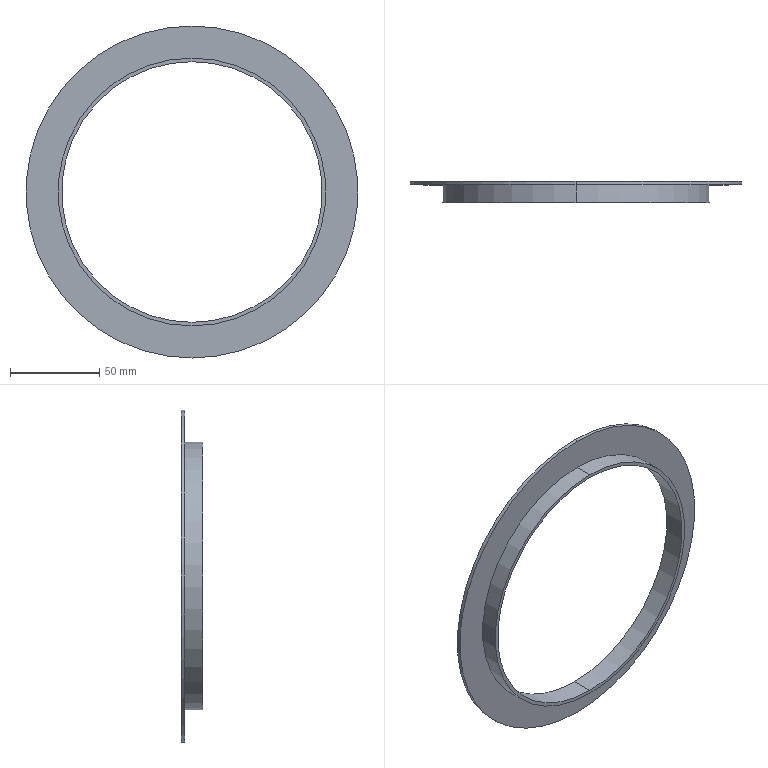Part | SolidWorks | features Extrusion 1, ICE 1 | 1 solid | 9 faces | box 186 x 12 x 186 mm | volume 30159 mm3 | cylinder 6 | plane 3 | commonest cylinder face diameters 146 x2 150 x2 186 x2
STEP:
#1=CARTESIAN_POINT('',(0.,12.,93.));
#2=VERTEX_POINT('',#1);
#3=CARTESIAN_POINT('',(0.,12.,-93.));
#4=VERTEX_POINT('',#3);
#5=CARTESIAN_POINT('',(0.,12.,0.));
#6=DIRECTION('',(0.,1.,0.));
#7=DIRECTION('',(0.,0.,1.));
#8=AXIS2_PLACEMENT_3D('',#5,#6,#7);
#9=CIRCLE('',#8,93.);
#10=EDGE_CURVE('',#2,#4,#9,.T.);
#11=ORIENTED_EDGE('',*,*,#10,.F.);
#12=CARTESIAN_POINT('',(0.,10.,93.));
#13=VERTEX_POINT('',#12);
#14=CARTESIAN_POINT('',(0.,12.,93.));
#15=DIRECTION('',(0.,-1.,0.));
#16=VECTOR('',#15,1000.);
#17=LINE('',#14,#16);
#18=EDGE_CURVE('',#2,#13,#17,.T.);
#19=ORIENTED_EDGE('',*,*,#18,.T.);
#20=CARTESIAN_POINT('',(0.,10.,-93.));
#21=VERTEX_POINT('',#20);
#22=CARTESIAN_POINT('',(0.,10.,0.));
#23=DIRECTION('',(0.,1.,0.));
#24=DIRECTION('',(0.,0.,1.));
#25=AXIS2_PLACEMENT_3D('',#22,#23,#24);
#26=CIRCLE('',#25,93.);
#27=EDGE_CURVE('',#13,#21,#26,.T.);
#28=ORIENTED_EDGE('',*,*,#27,.T.);
#29=CARTESIAN_POINT('',(0.,12.,-93.));
#30=DIRECTION('',(0.,-1.,0.));
#31=VECTOR('',#30,1000.);
#32=LINE('',#29,#31);
#33=EDGE_CURVE('',#4,#21,#32,.T.);
#34=ORIENTED_EDGE('',*,*,#33,.F.);
#35=EDGE_LOOP('',(#11,#19,#28,#34));
#36=FACE_OUTER_BOUND('',#35,.T.);
#37=CARTESIAN_POINT('',(0.,12.,0.));
#38=DIRECTION('',(0.,-1.,0.));
#39=DIRECTION('',(0.,0.,-1.));
#40=AXIS2_PLACEMENT_3D('',#37,#38,#39);
#41=CYLINDRICAL_SURFACE('',#40,93.);
#42=ADVANCED_FACE('',(#36),#41,.T.);
#43=CARTESIAN_POINT('',(0.,12.,-73.));
#44=VERTEX_POINT('',#43);
#45=CARTESIAN_POINT('',(0.,12.,73.));
#46=VERTEX_POINT('',#45);
#47=CARTESIAN_POINT('',(0.,12.,0.));
#48=DIRECTION('',(0.,1.,0.));
#49=DIRECTION('',(0.,0.,1.));
#50=AXIS2_PLACEMENT_3D('',#47,#48,#49);
#51=CIRCLE('',#50,73.);
#52=EDGE_CURVE('',#44,#46,#51,.T.);
#53=ORIENTED_EDGE('',*,*,#52,.T.);
#54=CARTESIAN_POINT('',(0.,0.,73.));
#55=VERTEX_POINT('',#54);
#56=CARTESIAN_POINT('',(0.,10.,73.));
#57=DIRECTION('',(0.,-1.,0.));
#58=VECTOR('',#57,1000.);
#59=LINE('',#56,#58);
#60=EDGE_CURVE('',#46,#55,#59,.T.);
#61=ORIENTED_EDGE('',*,*,#60,.T.);
#62=CARTESIAN_POINT('',(0.,0.,-73.));
#63=VERTEX_POINT('',#62);
#64=CARTESIAN_POINT('',(0.,0.,0.));
#65=DIRECTION('',(0.,1.,0.));
#66=DIRECTION('',(0.,0.,1.));
#67=AXIS2_PLACEMENT_3D('',#64,#65,#66);
#68=CIRCLE('',#67,73.);
#69=EDGE_CURVE('',#63,#55,#68,.T.);
#70=ORIENTED_EDGE('',*,*,#69,.F.);
#71=CARTESIAN_POINT('',(0.,10.,-73.));
#72=DIRECTION('',(0.,-1.,0.));
#73=VECTOR('',#72,1000.);
#74=LINE('',#71,#73);
#75=EDGE_CURVE('',#44,#63,#74,.T.);
#76=ORIENTED_EDGE('',*,*,#75,.F.);
#77=EDGE_LOOP('',(#53,#61,#70,#76));
#78=FACE_OUTER_BOUND('',#77,.T.);
#79=CARTESIAN_POINT('',(0.,10.,0.));
#80=DIRECTION('',(0.,-1.,0.));
#81=DIRECTION('',(0.,0.,-1.));
#82=AXIS2_PLACEMENT_3D('',#79,#80,#81);
#83=CYLINDRICAL_SURFACE('',#82,73.);
#84=ADVANCED_FACE('',(#78),#83,.F.);
#85=CARTESIAN_POINT('',(0.,10.,75.));
#86=VERTEX_POINT('',#85);
#87=CARTESIAN_POINT('',(0.,10.,-75.));
#88=VERTEX_POINT('',#87);
#89=CARTESIAN_POINT('',(0.,10.,0.));
#90=DIRECTION('',(0.,1.,0.));
#91=DIRECTION('',(0.,0.,1.));
#92=AXIS2_PLACEMENT_3D('',#89,#90,#91);
#93=CIRCLE('',#92,75.);
#94=EDGE_CURVE('',#86,#88,#93,.T.);
#95=ORIENTED_EDGE('',*,*,#94,.F.);
#96=CARTESIAN_POINT('',(0.,0.,75.));
#97=VERTEX_POINT('',#96);
#98=CARTESIAN_POINT('',(0.,10.,75.));
#99=DIRECTION('',(0.,-1.,0.));
#100=VECTOR('',#99,1000.);
#101=LINE('',#98,#100);
#102=EDGE_CURVE('',#86,#97,#101,.T.);
#103=ORIENTED_EDGE('',*,*,#102,.T.);
#104=CARTESIAN_POINT('',(0.,0.,-75.));
#105=VERTEX_POINT('',#104);
#106=CARTESIAN_POINT('',(0.,0.,0.));
#107=DIRECTION('',(0.,1.,0.));
#108=DIRECTION('',(0.,0.,1.));
#109=AXIS2_PLACEMENT_3D('',#106,#107,#108);
#110=CIRCLE('',#109,75.);
#111=EDGE_CURVE('',#97,#105,#110,.T.);
#112=ORIENTED_EDGE('',*,*,#111,.T.);
#113=CARTESIAN_POINT('',(0.,10.,-75.));
#114=DIRECTION('',(0.,-1.,0.));
#115=VECTOR('',#114,1000.);
#116=LINE('',#113,#115);
#117=EDGE_CURVE('',#88,#105,#116,.T.);
#118=ORIENTED_EDGE('',*,*,#117,.F.);
#119=EDGE_LOOP('',(#95,#103,#112,#118));
#120=FACE_OUTER_BOUND('',#119,.T.);
#121=CARTESIAN_POINT('',(0.,10.,0.));
#122=DIRECTION('',(0.,-1.,0.));
#123=DIRECTION('',(0.,0.,-1.));
#124=AXIS2_PLACEMENT_3D('',#121,#122,#123);
#125=CYLINDRICAL_SURFACE('',#124,75.);
#126=ADVANCED_FACE('',(#120),#125,.T.);
#127=CARTESIAN_POINT('',(0.,0.,0.));
#128=DIRECTION('',(0.,1.,0.));
#129=DIRECTION('',(0.,0.,1.));
#130=AXIS2_PLACEMENT_3D('',#127,#128,#129);
#131=CIRCLE('',#130,75.);
#132=EDGE_CURVE('',#105,#97,#131,.T.);
#133=ORIENTED_EDGE('',*,*,#132,.F.);
#134=ORIENTED_EDGE('',*,*,#111,.F.);
#135=EDGE_LOOP('',(#133,#134));
#136=FACE_OUTER_BOUND('',#135,.T.);
#137=ORIENTED_EDGE('',*,*,#69,.T.);
#138=CARTESIAN_POINT('',(0.,0.,0.));
#139=DIRECTION('',(0.,1.,0.));
#140=DIRECTION('',(0.,0.,1.));
#141=AXIS2_PLACEMENT_3D('',#138,#139,#140);
#142=CIRCLE('',#141,73.);
#143=EDGE_CURVE('',#55,#63,#142,.T.);
#144=ORIENTED_EDGE('',*,*,#143,.T.);
#145=EDGE_LOOP('',(#137,#144));
#146=FACE_BOUND('',#145,.T.);
#147=CARTESIAN_POINT('',(0.,0.,0.));
#148=DIRECTION('',(0.,1.,0.));
#149=DIRECTION('',(0.,0.,1.));
#150=AXIS2_PLACEMENT_3D('',#147,#148,#149);
#151=PLANE('',#150);
#152=ADVANCED_FACE('',(#136,#146),#151,.F.);
#153=ORIENTED_EDGE('',*,*,#102,.F.);
#154=CARTESIAN_POINT('',(0.,10.,0.));
#155=DIRECTION('',(0.,1.,0.));
#156=DIRECTION('',(0.,0.,1.));
#157=AXIS2_PLACEMENT_3D('',#154,#155,#156);
#158=CIRCLE('',#157,75.);
#159=EDGE_CURVE('',#88,#86,#158,.T.);
#160=ORIENTED_EDGE('',*,*,#159,.F.);
#161=ORIENTED_EDGE('',*,*,#117,.T.);
#162=ORIENTED_EDGE('',*,*,#132,.T.);
#163=EDGE_LOOP('',(#153,#160,#161,#162));
#164=FACE_OUTER_BOUND('',#163,.T.);
#165=CARTESIAN_POINT('',(0.,10.,0.));
#166=DIRECTION('',(0.,-1.,0.));
#167=DIRECTION('',(0.,0.,-1.));
#168=AXIS2_PLACEMENT_3D('',#165,#166,#167);
#169=CYLINDRICAL_SURFACE('',#168,75.);
#170=ADVANCED_FACE('',(#164),#169,.T.);
#171=ORIENTED_EDGE('',*,*,#60,.F.);
#172=CARTESIAN_POINT('',(0.,12.,0.));
#173=DIRECTION('',(0.,1.,0.));
#174=DIRECTION('',(0.,0.,1.));
#175=AXIS2_PLACEMENT_3D('',#172,#173,#174);
#176=CIRCLE('',#175,73.);
#177=EDGE_CURVE('',#46,#44,#176,.T.);
#178=ORIENTED_EDGE('',*,*,#177,.T.);
#179=ORIENTED_EDGE('',*,*,#75,.T.);
#180=ORIENTED_EDGE('',*,*,#143,.F.);
#181=EDGE_LOOP('',(#171,#178,#179,#180));
#182=FACE_OUTER_BOUND('',#181,.T.);
#183=CARTESIAN_POINT('',(0.,10.,0.));
#184=DIRECTION('',(0.,-1.,0.));
#185=DIRECTION('',(0.,0.,-1.));
#186=AXIS2_PLACEMENT_3D('',#183,#184,#185);
#187=CYLINDRICAL_SURFACE('',#186,73.);
#188=ADVANCED_FACE('',(#182),#187,.F.);
#189=CARTESIAN_POINT('',(0.,12.,0.));
#190=DIRECTION('',(0.,1.,0.));
#191=DIRECTION('',(0.,0.,1.));
#192=AXIS2_PLACEMENT_3D('',#189,#190,#191);
#193=CIRCLE('',#192,93.);
#194=EDGE_CURVE('',#4,#2,#193,.T.);
#195=ORIENTED_EDGE('',*,*,#194,.T.);
#196=ORIENTED_EDGE('',*,*,#10,.T.);
#197=EDGE_LOOP('',(#195,#196));
#198=FACE_OUTER_BOUND('',#197,.T.);
#199=ORIENTED_EDGE('',*,*,#52,.F.);
#200=ORIENTED_EDGE('',*,*,#177,.F.);
#201=EDGE_LOOP('',(#199,#200));
#202=FACE_BOUND('',#201,.T.);
#203=CARTESIAN_POINT('',(0.,12.,0.));
#204=DIRECTION('',(0.,1.,0.));
#205=DIRECTION('',(0.,0.,1.));
#206=AXIS2_PLACEMENT_3D('',#203,#204,#205);
#207=PLANE('',#206);
#208=ADVANCED_FACE('',(#198,#202),#207,.T.);
#209=ORIENTED_EDGE('',*,*,#159,.T.);
#210=ORIENTED_EDGE('',*,*,#94,.T.);
#211=EDGE_LOOP('',(#209,#210));
#212=FACE_BOUND('',#211,.T.);
#213=CARTESIAN_POINT('',(0.,10.,0.));
#214=DIRECTION('',(0.,1.,0.));
#215=DIRECTION('',(0.,0.,1.));
#216=AXIS2_PLACEMENT_3D('',#213,#214,#215);
#217=CIRCLE('',#216,93.);
#218=EDGE_CURVE('',#21,#13,#217,.T.);
#219=ORIENTED_EDGE('',*,*,#218,.F.);
#220=ORIENTED_EDGE('',*,*,#27,.F.);
#221=EDGE_LOOP('',(#219,#220));
#222=FACE_OUTER_BOUND('',#221,.T.);
#223=CARTESIAN_POINT('',(0.,10.,0.));
#224=DIRECTION('',(0.,1.,0.));
#225=DIRECTION('',(0.,0.,1.));
#226=AXIS2_PLACEMENT_3D('',#223,#224,#225);
#227=PLANE('',#226);
#228=ADVANCED_FACE('',(#212,#222),#227,.F.);
#229=ORIENTED_EDGE('',*,*,#18,.F.);
#230=ORIENTED_EDGE('',*,*,#194,.F.);
#231=ORIENTED_EDGE('',*,*,#33,.T.);
#232=ORIENTED_EDGE('',*,*,#218,.T.);
#233=EDGE_LOOP('',(#229,#230,#231,#232));
#234=FACE_OUTER_BOUND('',#233,.T.);
#235=CARTESIAN_POINT('',(0.,12.,0.));
#236=DIRECTION('',(0.,-1.,0.));
#237=DIRECTION('',(0.,0.,-1.));
#238=AXIS2_PLACEMENT_3D('',#235,#236,#237);
#239=CYLINDRICAL_SURFACE('',#238,93.);
#240=ADVANCED_FACE('',(#234),#239,.T.);
#241=CLOSED_SHELL('',(#42,#84,#126,#152,#170,#188,#208,#228,#240));
#242=MANIFOLD_SOLID_BREP('',#241);
#243=CARTESIAN_POINT('',(0.,0.,0.));
#244=DIRECTION('',(0.,0.,1.));
#245=DIRECTION('',(1.,0.,0.));
#246=AXIS2_PLACEMENT_3D('',#243,#244,#245);
#247=(LENGTH_UNIT()NAMED_UNIT(*)SI_UNIT(.MILLI.,.METRE.));
#248=UNCERTAINTY_MEASURE_WITH_UNIT(LENGTH_MEASURE(0.00001),#247,'','');
#249=(NAMED_UNIT(*)PLANE_ANGLE_UNIT()SI_UNIT($,.RADIAN.));
#250=(NAMED_UNIT(*)SI_UNIT($,.STERADIAN.)SOLID_ANGLE_UNIT());
#251=(GEOMETRIC_REPRESENTATION_CONTEXT(3)GLOBAL_UNCERTAINTY_ASSIGNED_CONTEXT((#248))GLOBAL_UNIT_ASSIGNED_CONTEXT((#247,#249,#250))REPRESENTATION_CONTEXT('',''));
#252=ADVANCED_BREP_SHAPE_REPRESENTATION('',(#242,#246),#251);